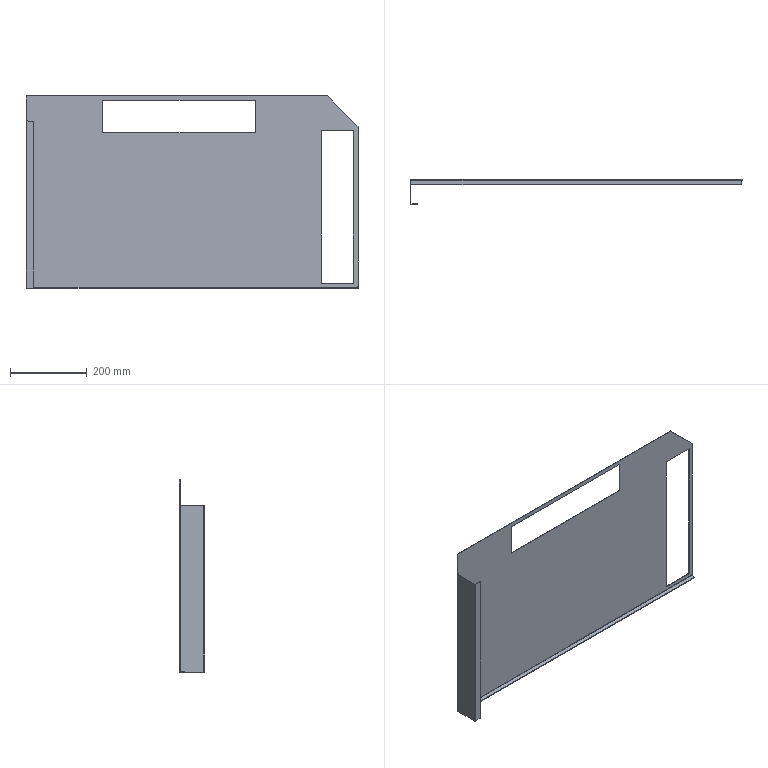Part | STEP file | Top Cover 2 | 1 solid | 39 faces | box 868 x 66 x 502.5 mm | volume 820735 mm3 | plane 30 | cylinder 9 | commonest cylinder face diameters 1 x6 5 x3
STEP:
#1=CARTESIAN_POINT('',(446.808,-2.,-297.25));
#2=VERTEX_POINT('',#1);
#3=CARTESIAN_POINT('',(447.308,-2.,-297.75));
#4=VERTEX_POINT('',#3);
#5=CARTESIAN_POINT('',(446.808,-2.,-297.75));
#6=DIRECTION('',(0.,1.,0.));
#7=DIRECTION('',(0.,0.,1.));
#8=AXIS2_PLACEMENT_3D('',#5,#6,#7);
#9=CIRCLE('',#8,0.5);
#10=EDGE_CURVE('',#2,#4,#9,.T.);
#11=ORIENTED_EDGE('',*,*,#10,.F.);
#12=CARTESIAN_POINT('',(446.808,0.,-297.25));
#13=VERTEX_POINT('',#12);
#14=CARTESIAN_POINT('',(446.808,-2.,-297.25));
#15=DIRECTION('',(0.,1.,0.));
#16=VECTOR('',#15,1000.);
#17=LINE('',#14,#16);
#18=EDGE_CURVE('',#2,#13,#17,.T.);
#19=ORIENTED_EDGE('',*,*,#18,.T.);
#20=CARTESIAN_POINT('',(447.308,0.,-297.75));
#21=VERTEX_POINT('',#20);
#22=CARTESIAN_POINT('',(446.808,0.,-297.75));
#23=DIRECTION('',(0.,-1.,0.));
#24=DIRECTION('',(0.,0.,1.));
#25=AXIS2_PLACEMENT_3D('',#22,#23,#24);
#26=CIRCLE('',#25,0.5);
#27=EDGE_CURVE('',#21,#13,#26,.T.);
#28=ORIENTED_EDGE('',*,*,#27,.F.);
#29=CARTESIAN_POINT('',(447.308,-2.,-297.75));
#30=DIRECTION('',(0.,1.,0.));
#31=VECTOR('',#30,1000.);
#32=LINE('',#29,#31);
#33=EDGE_CURVE('',#4,#21,#32,.T.);
#34=ORIENTED_EDGE('',*,*,#33,.F.);
#35=EDGE_LOOP('',(#11,#19,#28,#34));
#36=FACE_OUTER_BOUND('',#35,.T.);
#37=CARTESIAN_POINT('',(446.808,-2.,-297.75));
#38=DIRECTION('',(0.,1.,0.));
#39=DIRECTION('',(0.,0.,1.));
#40=AXIS2_PLACEMENT_3D('',#37,#38,#39);
#41=CYLINDRICAL_SURFACE('',#40,0.5);
#42=ADVANCED_FACE('',(#36),#41,.F.);
#43=ORIENTED_EDGE('',*,*,#27,.T.);
#44=CARTESIAN_POINT('',(446.308,0.,-297.75));
#45=VERTEX_POINT('',#44);
#46=CARTESIAN_POINT('',(446.808,0.,-297.75));
#47=DIRECTION('',(0.,-1.,0.));
#48=DIRECTION('',(0.,0.,1.));
#49=AXIS2_PLACEMENT_3D('',#46,#47,#48);
#50=CIRCLE('',#49,0.5);
#51=EDGE_CURVE('',#13,#45,#50,.T.);
#52=ORIENTED_EDGE('',*,*,#51,.T.);
#53=CARTESIAN_POINT('',(446.308,0.,-298.75));
#54=VERTEX_POINT('',#53);
#55=CARTESIAN_POINT('',(446.308,0.,-297.75));
#56=DIRECTION('',(0.,0.,1.));
#57=VECTOR('',#56,1000.);
#58=LINE('',#55,#57);
#59=EDGE_CURVE('',#54,#45,#58,.T.);
#60=ORIENTED_EDGE('',*,*,#59,.F.);
#61=CARTESIAN_POINT('',(-417.192,0.,-298.75));
#62=VERTEX_POINT('',#61);
#63=CARTESIAN_POINT('',(0.,0.,-298.75));
#64=DIRECTION('',(1.,0.,0.));
#65=VECTOR('',#64,1000.);
#66=LINE('',#63,#65);
#67=EDGE_CURVE('',#62,#54,#66,.T.);
#68=ORIENTED_EDGE('',*,*,#67,.F.);
#69=CARTESIAN_POINT('',(-417.192,0.,135.25));
#70=VERTEX_POINT('',#69);
#71=CARTESIAN_POINT('',(-417.192,0.,0.));
#72=DIRECTION('',(0.,0.,-1.));
#73=VECTOR('',#72,1000.);
#74=LINE('',#71,#73);
#75=EDGE_CURVE('',#70,#62,#74,.T.);
#76=ORIENTED_EDGE('',*,*,#75,.F.);
#77=CARTESIAN_POINT('',(-416.192,0.,135.25));
#78=VERTEX_POINT('',#77);
#79=CARTESIAN_POINT('',(-417.192,0.,135.25));
#80=DIRECTION('',(-1.,0.,0.));
#81=VECTOR('',#80,1000.);
#82=LINE('',#79,#81);
#83=EDGE_CURVE('',#78,#70,#82,.T.);
#84=ORIENTED_EDGE('',*,*,#83,.F.);
#85=CARTESIAN_POINT('',(-416.192,0.,136.25));
#86=VERTEX_POINT('',#85);
#87=CARTESIAN_POINT('',(-416.192,0.,135.75));
#88=DIRECTION('',(0.,-1.,0.));
#89=DIRECTION('',(0.,0.,1.));
#90=AXIS2_PLACEMENT_3D('',#87,#88,#89);
#91=CIRCLE('',#90,0.5);
#92=EDGE_CURVE('',#78,#86,#91,.T.);
#93=ORIENTED_EDGE('',*,*,#92,.T.);
#94=CARTESIAN_POINT('',(-419.692,0.,136.25));
#95=VERTEX_POINT('',#94);
#96=CARTESIAN_POINT('',(0.,0.,136.25));
#97=DIRECTION('',(1.,0.,0.));
#98=VECTOR('',#97,1000.);
#99=LINE('',#96,#98);
#100=EDGE_CURVE('',#95,#86,#99,.T.);
#101=ORIENTED_EDGE('',*,*,#100,.F.);
#102=CARTESIAN_POINT('',(-419.692,0.,201.25));
#103=VERTEX_POINT('',#102);
#104=CARTESIAN_POINT('',(-419.692,0.,0.));
#105=DIRECTION('',(0.,0.,-1.));
#106=VECTOR('',#105,1000.);
#107=LINE('',#104,#106);
#108=EDGE_CURVE('',#103,#95,#107,.T.);
#109=ORIENTED_EDGE('',*,*,#108,.F.);
#110=CARTESIAN_POINT('',(368.308,0.,201.25));
#111=VERTEX_POINT('',#110);
#112=CARTESIAN_POINT('',(0.,0.,201.25));
#113=DIRECTION('',(-1.,0.,0.));
#114=VECTOR('',#113,1000.);
#115=LINE('',#112,#114);
#116=EDGE_CURVE('',#111,#103,#115,.T.);
#117=ORIENTED_EDGE('',*,*,#116,.F.);
#118=CARTESIAN_POINT('',(448.308,0.,121.25));
#119=VERTEX_POINT('',#118);
#120=CARTESIAN_POINT('',(448.308,0.,121.25));
#121=DIRECTION('',(-0.7071,0.,0.7071));
#122=VECTOR('',#121,1000.);
#123=LINE('',#120,#122);
#124=EDGE_CURVE('',#119,#111,#123,.T.);
#125=ORIENTED_EDGE('',*,*,#124,.F.);
#126=CARTESIAN_POINT('',(448.308,0.,-301.25));
#127=VERTEX_POINT('',#126);
#128=CARTESIAN_POINT('',(448.308,0.,0.));
#129=DIRECTION('',(0.,0.,1.));
#130=VECTOR('',#129,1000.);
#131=LINE('',#128,#130);
#132=EDGE_CURVE('',#127,#119,#131,.T.);
#133=ORIENTED_EDGE('',*,*,#132,.F.);
#134=CARTESIAN_POINT('',(447.308,0.,-301.25));
#135=VERTEX_POINT('',#134);
#136=CARTESIAN_POINT('',(448.308,0.,-301.25));
#137=DIRECTION('',(1.,0.,0.));
#138=VECTOR('',#137,1000.);
#139=LINE('',#136,#138);
#140=EDGE_CURVE('',#135,#127,#139,.T.);
#141=ORIENTED_EDGE('',*,*,#140,.F.);
#142=CARTESIAN_POINT('',(447.308,0.,0.));
#143=DIRECTION('',(0.,0.,-1.));
#144=VECTOR('',#143,1000.);
#145=LINE('',#142,#144);
#146=EDGE_CURVE('',#21,#135,#145,.T.);
#147=ORIENTED_EDGE('',*,*,#146,.F.);
#148=EDGE_LOOP('',(#43,#52,#60,#68,#76,#84,#93,#101,#109,#117,#125,#133,#141,#147));
#149=FACE_OUTER_BOUND('',#148,.T.);
#150=CARTESIAN_POINT('',(-219.692,0.,105.25));
#151=VERTEX_POINT('',#150);
#152=CARTESIAN_POINT('',(-219.692,0.,189.25));
#153=VERTEX_POINT('',#152);
#154=CARTESIAN_POINT('',(-219.692,0.,0.));
#155=DIRECTION('',(0.,0.,1.));
#156=VECTOR('',#155,1000.);
#157=LINE('',#154,#156);
#158=EDGE_CURVE('',#151,#153,#157,.T.);
#159=ORIENTED_EDGE('',*,*,#158,.F.);
#160=CARTESIAN_POINT('',(180.308,0.,105.25));
#161=VERTEX_POINT('',#160);
#162=CARTESIAN_POINT('',(0.,0.,105.25));
#163=DIRECTION('',(-1.,0.,0.));
#164=VECTOR('',#163,1000.);
#165=LINE('',#162,#164);
#166=EDGE_CURVE('',#161,#151,#165,.T.);
#167=ORIENTED_EDGE('',*,*,#166,.F.);
#168=CARTESIAN_POINT('',(180.308,0.,189.25));
#169=VERTEX_POINT('',#168);
#170=CARTESIAN_POINT('',(180.308,0.,0.));
#171=DIRECTION('',(0.,0.,-1.));
#172=VECTOR('',#171,1000.);
#173=LINE('',#170,#172);
#174=EDGE_CURVE('',#169,#161,#173,.T.);
#175=ORIENTED_EDGE('',*,*,#174,.F.);
#176=CARTESIAN_POINT('',(0.,0.,189.25));
#177=DIRECTION('',(1.,0.,0.));
#178=VECTOR('',#177,1000.);
#179=LINE('',#176,#178);
#180=EDGE_CURVE('',#153,#169,#179,.T.);
#181=ORIENTED_EDGE('',*,*,#180,.F.);
#182=EDGE_LOOP('',(#159,#167,#175,#181));
#183=FACE_BOUND('',#182,.T.);
#184=CARTESIAN_POINT('',(352.308,0.,-288.75));
#185=VERTEX_POINT('',#184);
#186=CARTESIAN_POINT('',(352.308,0.,111.25));
#187=VERTEX_POINT('',#186);
#188=CARTESIAN_POINT('',(352.308,0.,0.));
#189=DIRECTION('',(0.,0.,1.));
#190=VECTOR('',#189,1000.);
#191=LINE('',#188,#190);
#192=EDGE_CURVE('',#185,#187,#191,.T.);
#193=ORIENTED_EDGE('',*,*,#192,.F.);
#194=CARTESIAN_POINT('',(436.308,0.,-288.75));
#195=VERTEX_POINT('',#194);
#196=CARTESIAN_POINT('',(0.,0.,-288.75));
#197=DIRECTION('',(-1.,0.,0.));
#198=VECTOR('',#197,1000.);
#199=LINE('',#196,#198);
#200=EDGE_CURVE('',#195,#185,#199,.T.);
#201=ORIENTED_EDGE('',*,*,#200,.F.);
#202=CARTESIAN_POINT('',(436.308,0.,111.25));
#203=VERTEX_POINT('',#202);
#204=CARTESIAN_POINT('',(436.308,0.,0.));
#205=DIRECTION('',(0.,0.,-1.));
#206=VECTOR('',#205,1000.);
#207=LINE('',#204,#206);
#208=EDGE_CURVE('',#203,#195,#207,.T.);
#209=ORIENTED_EDGE('',*,*,#208,.F.);
#210=CARTESIAN_POINT('',(0.,0.,111.25));
#211=DIRECTION('',(1.,0.,0.));
#212=VECTOR('',#211,1000.);
#213=LINE('',#210,#212);
#214=EDGE_CURVE('',#187,#203,#213,.T.);
#215=ORIENTED_EDGE('',*,*,#214,.F.);
#216=EDGE_LOOP('',(#193,#201,#209,#215));
#217=FACE_BOUND('',#216,.T.);
#218=CARTESIAN_POINT('',(0.,0.,0.));
#219=DIRECTION('',(0.,-1.,0.));
#220=DIRECTION('',(0.,0.,-1.));
#221=AXIS2_PLACEMENT_3D('',#218,#219,#220);
#222=PLANE('',#221);
#223=ADVANCED_FACE('',(#149,#183,#217),#222,.F.);
#224=CARTESIAN_POINT('',(447.308,-2.,-301.25));
#225=VERTEX_POINT('',#224);
#226=CARTESIAN_POINT('',(447.308,-2.,-301.25));
#227=DIRECTION('',(0.,-1.,0.));
#228=VECTOR('',#227,1000.);
#229=LINE('',#226,#228);
#230=EDGE_CURVE('',#135,#225,#229,.T.);
#231=ORIENTED_EDGE('',*,*,#230,.T.);
#232=CARTESIAN_POINT('',(447.308,-2.,-301.25));
#233=DIRECTION('',(0.,0.,1.));
#234=VECTOR('',#233,1000.);
#235=LINE('',#232,#234);
#236=EDGE_CURVE('',#225,#4,#235,.T.);
#237=ORIENTED_EDGE('',*,*,#236,.T.);
#238=ORIENTED_EDGE('',*,*,#33,.T.);
#239=ORIENTED_EDGE('',*,*,#146,.T.);
#240=EDGE_LOOP('',(#231,#237,#238,#239));
#241=FACE_OUTER_BOUND('',#240,.T.);
#242=CARTESIAN_POINT('',(447.308,-2.,-301.25));
#243=DIRECTION('',(-1.,0.,0.));
#244=DIRECTION('',(0.,0.,1.));
#245=AXIS2_PLACEMENT_3D('',#242,#243,#244);
#246=PLANE('',#245);
#247=ADVANCED_FACE('',(#241),#246,.T.);
#248=CARTESIAN_POINT('',(-417.192,-2.,-301.199));
#249=VERTEX_POINT('',#248);
#250=CARTESIAN_POINT('',(-417.192,-2.5,-301.25));
#251=VERTEX_POINT('',#250);
#252=CARTESIAN_POINT('',(-417.192,-2.5,-298.75));
#253=DIRECTION('',(-1.,0.,0.));
#254=DIRECTION('',(0.,0.,-1.));
#255=AXIS2_PLACEMENT_3D('',#252,#253,#254);
#256=CIRCLE('',#255,2.5);
#257=EDGE_CURVE('',#249,#251,#256,.T.);
#258=ORIENTED_EDGE('',*,*,#257,.F.);
#259=CARTESIAN_POINT('',(-417.192,-2.5,-298.75));
#260=DIRECTION('',(1.,0.,0.));
#261=DIRECTION('',(0.,0.,-1.));
#262=AXIS2_PLACEMENT_3D('',#259,#260,#261);
#263=CIRCLE('',#262,2.5);
#264=EDGE_CURVE('',#249,#62,#263,.T.);
#265=ORIENTED_EDGE('',*,*,#264,.T.);
#266=ORIENTED_EDGE('',*,*,#67,.T.);
#267=CARTESIAN_POINT('',(446.308,-2.5,-301.25));
#268=VERTEX_POINT('',#267);
#269=CARTESIAN_POINT('',(446.308,-2.5,-298.75));
#270=DIRECTION('',(-1.,0.,0.));
#271=DIRECTION('',(0.,0.,-1.));
#272=AXIS2_PLACEMENT_3D('',#269,#270,#271);
#273=CIRCLE('',#272,2.5);
#274=EDGE_CURVE('',#54,#268,#273,.T.);
#275=ORIENTED_EDGE('',*,*,#274,.T.);
#276=CARTESIAN_POINT('',(446.308,-2.5,-301.25));
#277=DIRECTION('',(-1.,0.,0.));
#278=VECTOR('',#277,1000.);
#279=LINE('',#276,#278);
#280=EDGE_CURVE('',#268,#251,#279,.T.);
#281=ORIENTED_EDGE('',*,*,#280,.T.);
#282=EDGE_LOOP('',(#258,#265,#266,#275,#281));
#283=FACE_OUTER_BOUND('',#282,.T.);
#284=CARTESIAN_POINT('',(446.308,-2.5,-298.75));
#285=DIRECTION('',(1.,0.,0.));
#286=DIRECTION('',(0.,0.,-1.));
#287=AXIS2_PLACEMENT_3D('',#284,#285,#286);
#288=CYLINDRICAL_SURFACE('',#287,2.5);
#289=ADVANCED_FACE('',(#283),#288,.T.);
#290=CARTESIAN_POINT('',(-419.692,-2.5,135.25));
#291=VERTEX_POINT('',#290);
#292=CARTESIAN_POINT('',(-417.192,-2.5,135.25));
#293=DIRECTION('',(0.,0.,-1.));
#294=DIRECTION('',(-1.,0.,0.));
#295=AXIS2_PLACEMENT_3D('',#292,#293,#294);
#296=CIRCLE('',#295,2.5);
#297=EDGE_CURVE('',#291,#70,#296,.T.);
#298=ORIENTED_EDGE('',*,*,#297,.T.);
#299=ORIENTED_EDGE('',*,*,#75,.T.);
#300=CARTESIAN_POINT('',(-417.192,0.,-301.25));
#301=VERTEX_POINT('',#300);
#302=CARTESIAN_POINT('',(-417.192,0.,-301.25));
#303=DIRECTION('',(0.,0.,-1.));
#304=VECTOR('',#303,1000.);
#305=LINE('',#302,#304);
#306=EDGE_CURVE('',#62,#301,#305,.T.);
#307=ORIENTED_EDGE('',*,*,#306,.T.);
#308=CARTESIAN_POINT('',(-419.692,-2.5,-301.25));
#309=VERTEX_POINT('',#308);
#310=CARTESIAN_POINT('',(-417.192,-2.5,-301.25));
#311=DIRECTION('',(0.,0.,1.));
#312=DIRECTION('',(-1.,0.,0.));
#313=AXIS2_PLACEMENT_3D('',#310,#311,#312);
#314=CIRCLE('',#313,2.5);
#315=EDGE_CURVE('',#301,#309,#314,.T.);
#316=ORIENTED_EDGE('',*,*,#315,.T.);
#317=CARTESIAN_POINT('',(-419.692,-2.5,-301.25));
#318=DIRECTION('',(0.,0.,1.));
#319=VECTOR('',#318,1000.);
#320=LINE('',#317,#319);
#321=EDGE_CURVE('',#309,#291,#320,.T.);
#322=ORIENTED_EDGE('',*,*,#321,.T.);
#323=EDGE_LOOP('',(#298,#299,#307,#316,#322));
#324=FACE_OUTER_BOUND('',#323,.T.);
#325=CARTESIAN_POINT('',(-417.192,-2.5,-301.25));
#326=DIRECTION('',(0.,0.,-1.));
#327=DIRECTION('',(-1.,0.,0.));
#328=AXIS2_PLACEMENT_3D('',#325,#326,#327);
#329=CYLINDRICAL_SURFACE('',#328,2.5);
#330=ADVANCED_FACE('',(#324),#329,.T.);
#331=CARTESIAN_POINT('',(-416.192,-2.,136.25));
#332=VERTEX_POINT('',#331);
#333=CARTESIAN_POINT('',(-416.192,-2.,136.25));
#334=DIRECTION('',(0.,-1.,0.));
#335=VECTOR('',#334,1000.);
#336=LINE('',#333,#335);
#337=EDGE_CURVE('',#86,#332,#336,.T.);
#338=ORIENTED_EDGE('',*,*,#337,.T.);
#339=CARTESIAN_POINT('',(-419.692,-2.,136.25));
#340=VERTEX_POINT('',#339);
#341=CARTESIAN_POINT('',(-416.192,-2.,136.25));
#342=DIRECTION('',(-1.,0.,0.));
#343=VECTOR('',#342,1000.);
#344=LINE('',#341,#343);
#345=EDGE_CURVE('',#332,#340,#344,.T.);
#346=ORIENTED_EDGE('',*,*,#345,.T.);
#347=CARTESIAN_POINT('',(-419.692,-2.,136.25));
#348=DIRECTION('',(0.,1.,0.));
#349=VECTOR('',#348,1000.);
#350=LINE('',#347,#349);
#351=EDGE_CURVE('',#340,#95,#350,.T.);
#352=ORIENTED_EDGE('',*,*,#351,.T.);
#353=ORIENTED_EDGE('',*,*,#100,.T.);
#354=EDGE_LOOP('',(#338,#346,#352,#353));
#355=FACE_OUTER_BOUND('',#354,.T.);
#356=CARTESIAN_POINT('',(-416.192,-2.,136.25));
#357=DIRECTION('',(0.,0.,-1.));
#358=DIRECTION('',(0.,1.,0.));
#359=AXIS2_PLACEMENT_3D('',#356,#357,#358);
#360=PLANE('',#359);
#361=ADVANCED_FACE('',(#355),#360,.T.);
#362=CARTESIAN_POINT('',(-419.692,-2.,201.25));
#363=VERTEX_POINT('',#362);
#364=CARTESIAN_POINT('',(-419.692,-2.,-301.25));
#365=DIRECTION('',(0.,0.,1.));
#366=VECTOR('',#365,1000.);
#367=LINE('',#364,#366);
#368=EDGE_CURVE('',#340,#363,#367,.T.);
#369=ORIENTED_EDGE('',*,*,#368,.T.);
#370=CARTESIAN_POINT('',(-419.692,-2.,201.25));
#371=DIRECTION('',(0.,1.,0.));
#372=VECTOR('',#371,1000.);
#373=LINE('',#370,#372);
#374=EDGE_CURVE('',#363,#103,#373,.T.);
#375=ORIENTED_EDGE('',*,*,#374,.T.);
#376=ORIENTED_EDGE('',*,*,#108,.T.);
#377=ORIENTED_EDGE('',*,*,#351,.F.);
#378=EDGE_LOOP('',(#369,#375,#376,#377));
#379=FACE_OUTER_BOUND('',#378,.T.);
#380=CARTESIAN_POINT('',(-419.692,-2.,-301.25));
#381=DIRECTION('',(-1.,0.,0.));
#382=DIRECTION('',(0.,0.,1.));
#383=AXIS2_PLACEMENT_3D('',#380,#381,#382);
#384=PLANE('',#383);
#385=ADVANCED_FACE('',(#379),#384,.T.);
#386=CARTESIAN_POINT('',(368.308,-2.,201.25));
#387=VERTEX_POINT('',#386);
#388=CARTESIAN_POINT('',(368.308,-2.,201.25));
#389=DIRECTION('',(1.,0.,0.));
#390=VECTOR('',#389,1000.);
#391=LINE('',#388,#390);
#392=EDGE_CURVE('',#363,#387,#391,.T.);
#393=ORIENTED_EDGE('',*,*,#392,.T.);
#394=CARTESIAN_POINT('',(368.308,-2.,201.25));
#395=DIRECTION('',(0.,1.,0.));
#396=VECTOR('',#395,1000.);
#397=LINE('',#394,#396);
#398=EDGE_CURVE('',#387,#111,#397,.T.);
#399=ORIENTED_EDGE('',*,*,#398,.T.);
#400=ORIENTED_EDGE('',*,*,#116,.T.);
#401=ORIENTED_EDGE('',*,*,#374,.F.);
#402=EDGE_LOOP('',(#393,#399,#400,#401));
#403=FACE_OUTER_BOUND('',#402,.T.);
#404=CARTESIAN_POINT('',(368.308,-2.,201.25));
#405=DIRECTION('',(0.,0.,1.));
#406=DIRECTION('',(1.,0.,0.));
#407=AXIS2_PLACEMENT_3D('',#404,#405,#406);
#408=PLANE('',#407);
#409=ADVANCED_FACE('',(#403),#408,.T.);
#410=CARTESIAN_POINT('',(448.308,-2.,121.25));
#411=VERTEX_POINT('',#410);
#412=CARTESIAN_POINT('',(448.308,-2.,121.25));
#413=DIRECTION('',(0.7071,0.,-0.7071));
#414=VECTOR('',#413,1000.);
#415=LINE('',#412,#414);
#416=EDGE_CURVE('',#387,#411,#415,.T.);
#417=ORIENTED_EDGE('',*,*,#416,.T.);
#418=CARTESIAN_POINT('',(448.308,-2.,121.25));
#419=DIRECTION('',(0.,1.,0.));
#420=VECTOR('',#419,1000.);
#421=LINE('',#418,#420);
#422=EDGE_CURVE('',#411,#119,#421,.T.);
#423=ORIENTED_EDGE('',*,*,#422,.T.);
#424=ORIENTED_EDGE('',*,*,#124,.T.);
#425=ORIENTED_EDGE('',*,*,#398,.F.);
#426=EDGE_LOOP('',(#417,#423,#424,#425));
#427=FACE_OUTER_BOUND('',#426,.T.);
#428=CARTESIAN_POINT('',(448.308,-2.,121.25));
#429=DIRECTION('',(0.7071,0.,0.7071));
#430=DIRECTION('',(0.7071,0.,-0.7071));
#431=AXIS2_PLACEMENT_3D('',#428,#429,#430);
#432=PLANE('',#431);
#433=ADVANCED_FACE('',(#427),#432,.T.);
#434=CARTESIAN_POINT('',(448.308,-2.,-301.25));
#435=VERTEX_POINT('',#434);
#436=CARTESIAN_POINT('',(448.308,-2.,-301.25));
#437=DIRECTION('',(0.,0.,-1.));
#438=VECTOR('',#437,1000.);
#439=LINE('',#436,#438);
#440=EDGE_CURVE('',#411,#435,#439,.T.);
#441=ORIENTED_EDGE('',*,*,#440,.T.);
#442=CARTESIAN_POINT('',(448.308,-2.,-301.25));
#443=DIRECTION('',(0.,1.,0.));
#444=VECTOR('',#443,1000.);
#445=LINE('',#442,#444);
#446=EDGE_CURVE('',#435,#127,#445,.T.);
#447=ORIENTED_EDGE('',*,*,#446,.T.);
#448=ORIENTED_EDGE('',*,*,#132,.T.);
#449=ORIENTED_EDGE('',*,*,#422,.F.);
#450=EDGE_LOOP('',(#441,#447,#448,#449));
#451=FACE_OUTER_BOUND('',#450,.T.);
#452=CARTESIAN_POINT('',(448.308,-2.,-301.25));
#453=DIRECTION('',(1.,0.,0.));
#454=DIRECTION('',(0.,0.,-1.));
#455=AXIS2_PLACEMENT_3D('',#452,#453,#454);
#456=PLANE('',#455);
#457=ADVANCED_FACE('',(#451),#456,.T.);
#458=CARTESIAN_POINT('',(-219.692,-2.,189.25));
#459=VERTEX_POINT('',#458);
#460=CARTESIAN_POINT('',(-219.692,-10.,189.25));
#461=DIRECTION('',(0.,-1.,0.));
#462=VECTOR('',#461,1000.);
#463=LINE('',#460,#462);
#464=EDGE_CURVE('',#153,#459,#463,.T.);
#465=ORIENTED_EDGE('',*,*,#464,.F.);
#466=ORIENTED_EDGE('',*,*,#180,.T.);
#467=CARTESIAN_POINT('',(180.308,-2.,189.25));
#468=VERTEX_POINT('',#467);
#469=CARTESIAN_POINT('',(180.308,-10.,189.25));
#470=DIRECTION('',(0.,1.,0.));
#471=VECTOR('',#470,1000.);
#472=LINE('',#469,#471);
#473=EDGE_CURVE('',#468,#169,#472,.T.);
#474=ORIENTED_EDGE('',*,*,#473,.F.);
#475=CARTESIAN_POINT('',(-219.692,-2.,189.25));
#476=DIRECTION('',(1.,0.,0.));
#477=VECTOR('',#476,1000.);
#478=LINE('',#475,#477);
#479=EDGE_CURVE('',#459,#468,#478,.T.);
#480=ORIENTED_EDGE('',*,*,#479,.F.);
#481=EDGE_LOOP('',(#465,#466,#474,#480));
#482=FACE_OUTER_BOUND('',#481,.T.);
#483=CARTESIAN_POINT('',(-219.692,-10.,189.25));
#484=DIRECTION('',(0.,0.,1.));
#485=DIRECTION('',(1.,0.,0.));
#486=AXIS2_PLACEMENT_3D('',#483,#484,#485);
#487=PLANE('',#486);
#488=ADVANCED_FACE('',(#482),#487,.F.);
#489=CARTESIAN_POINT('',(-219.692,-2.,105.25));
#490=VERTEX_POINT('',#489);
#491=CARTESIAN_POINT('',(-219.692,-10.,105.25));
#492=DIRECTION('',(0.,-1.,0.));
#493=VECTOR('',#492,1000.);
#494=LINE('',#491,#493);
#495=EDGE_CURVE('',#151,#490,#494,.T.);
#496=ORIENTED_EDGE('',*,*,#495,.F.);
#497=ORIENTED_EDGE('',*,*,#158,.T.);
#498=ORIENTED_EDGE('',*,*,#464,.T.);
#499=CARTESIAN_POINT('',(-219.692,-2.,105.25));
#500=DIRECTION('',(0.,0.,1.));
#501=VECTOR('',#500,1000.);
#502=LINE('',#499,#501);
#503=EDGE_CURVE('',#490,#459,#502,.T.);
#504=ORIENTED_EDGE('',*,*,#503,.F.);
#505=EDGE_LOOP('',(#496,#497,#498,#504));
#506=FACE_OUTER_BOUND('',#505,.T.);
#507=CARTESIAN_POINT('',(-219.692,-10.,105.25));
#508=DIRECTION('',(-1.,0.,0.));
#509=DIRECTION('',(0.,0.,1.));
#510=AXIS2_PLACEMENT_3D('',#507,#508,#509);
#511=PLANE('',#510);
#512=ADVANCED_FACE('',(#506),#511,.F.);
#513=CARTESIAN_POINT('',(180.308,-2.,105.25));
#514=VERTEX_POINT('',#513);
#515=CARTESIAN_POINT('',(180.308,-10.,105.25));
#516=DIRECTION('',(0.,-1.,0.));
#517=VECTOR('',#516,1000.);
#518=LINE('',#515,#517);
#519=EDGE_CURVE('',#161,#514,#518,.T.);
#520=ORIENTED_EDGE('',*,*,#519,.F.);
#521=ORIENTED_EDGE('',*,*,#166,.T.);
#522=ORIENTED_EDGE('',*,*,#495,.T.);
#523=CARTESIAN_POINT('',(-219.692,-2.,105.25));
#524=DIRECTION('',(-1.,0.,0.));
#525=VECTOR('',#524,1000.);
#526=LINE('',#523,#525);
#527=EDGE_CURVE('',#514,#490,#526,.T.);
#528=ORIENTED_EDGE('',*,*,#527,.F.);
#529=EDGE_LOOP('',(#520,#521,#522,#528));
#530=FACE_OUTER_BOUND('',#529,.T.);
#531=CARTESIAN_POINT('',(-219.692,-10.,105.25));
#532=DIRECTION('',(0.,0.,-1.));
#533=DIRECTION('',(-1.,0.,0.));
#534=AXIS2_PLACEMENT_3D('',#531,#532,#533);
#535=PLANE('',#534);
#536=ADVANCED_FACE('',(#530),#535,.F.);
#537=ORIENTED_EDGE('',*,*,#473,.T.);
#538=ORIENTED_EDGE('',*,*,#174,.T.);
#539=ORIENTED_EDGE('',*,*,#519,.T.);
#540=CARTESIAN_POINT('',(180.308,-2.,105.25));
#541=DIRECTION('',(0.,0.,-1.));
#542=VECTOR('',#541,1000.);
#543=LINE('',#540,#542);
#544=EDGE_CURVE('',#468,#514,#543,.T.);
#545=ORIENTED_EDGE('',*,*,#544,.F.);
#546=EDGE_LOOP('',(#537,#538,#539,#545));
#547=FACE_OUTER_BOUND('',#546,.T.);
#548=CARTESIAN_POINT('',(180.308,-10.,105.25));
#549=DIRECTION('',(1.,0.,0.));
#550=DIRECTION('',(0.,0.,-1.));
#551=AXIS2_PLACEMENT_3D('',#548,#549,#550);
#552=PLANE('',#551);
#553=ADVANCED_FACE('',(#547),#552,.F.);
#554=CARTESIAN_POINT('',(352.308,-2.,111.25));
#555=VERTEX_POINT('',#554);
#556=CARTESIAN_POINT('',(352.308,-10.,111.25));
#557=DIRECTION('',(0.,-1.,0.));
#558=VECTOR('',#557,1000.);
#559=LINE('',#556,#558);
#560=EDGE_CURVE('',#187,#555,#559,.T.);
#561=ORIENTED_EDGE('',*,*,#560,.F.);
#562=ORIENTED_EDGE('',*,*,#214,.T.);
#563=CARTESIAN_POINT('',(436.308,-2.,111.25));
#564=VERTEX_POINT('',#563);
#565=CARTESIAN_POINT('',(436.308,-10.,111.25));
#566=DIRECTION('',(0.,1.,0.));
#567=VECTOR('',#566,1000.);
#568=LINE('',#565,#567);
#569=EDGE_CURVE('',#564,#203,#568,.T.);
#570=ORIENTED_EDGE('',*,*,#569,.F.);
#571=CARTESIAN_POINT('',(352.308,-2.,111.25));
#572=DIRECTION('',(1.,0.,0.));
#573=VECTOR('',#572,1000.);
#574=LINE('',#571,#573);
#575=EDGE_CURVE('',#555,#564,#574,.T.);
#576=ORIENTED_EDGE('',*,*,#575,.F.);
#577=EDGE_LOOP('',(#561,#562,#570,#576));
#578=FACE_OUTER_BOUND('',#577,.T.);
#579=CARTESIAN_POINT('',(352.308,-10.,111.25));
#580=DIRECTION('',(0.,0.,1.));
#581=DIRECTION('',(1.,0.,0.));
#582=AXIS2_PLACEMENT_3D('',#579,#580,#581);
#583=PLANE('',#582);
#584=ADVANCED_FACE('',(#578),#583,.F.);
#585=CARTESIAN_POINT('',(352.308,-2.,-288.75));
#586=VERTEX_POINT('',#585);
#587=CARTESIAN_POINT('',(352.308,-10.,-288.75));
#588=DIRECTION('',(0.,-1.,0.));
#589=VECTOR('',#588,1000.);
#590=LINE('',#587,#589);
#591=EDGE_CURVE('',#185,#586,#590,.T.);
#592=ORIENTED_EDGE('',*,*,#591,.F.);
#593=ORIENTED_EDGE('',*,*,#192,.T.);
#594=ORIENTED_EDGE('',*,*,#560,.T.);
#595=CARTESIAN_POINT('',(352.308,-2.,-288.75));
#596=DIRECTION('',(0.,0.,1.));
#597=VECTOR('',#596,1000.);
#598=LINE('',#595,#597);
#599=EDGE_CURVE('',#586,#555,#598,.T.);
#600=ORIENTED_EDGE('',*,*,#599,.F.);
#601=EDGE_LOOP('',(#592,#593,#594,#600));
#602=FACE_OUTER_BOUND('',#601,.T.);
#603=CARTESIAN_POINT('',(352.308,-10.,-288.75));
#604=DIRECTION('',(-1.,0.,0.));
#605=DIRECTION('',(0.,0.,1.));
#606=AXIS2_PLACEMENT_3D('',#603,#604,#605);
#607=PLANE('',#606);
#608=ADVANCED_FACE('',(#602),#607,.F.);
#609=CARTESIAN_POINT('',(436.308,-2.,-288.75));
#610=VERTEX_POINT('',#609);
#611=CARTESIAN_POINT('',(436.308,-10.,-288.75));
#612=DIRECTION('',(0.,-1.,0.));
#613=VECTOR('',#612,1000.);
#614=LINE('',#611,#613);
#615=EDGE_CURVE('',#195,#610,#614,.T.);
#616=ORIENTED_EDGE('',*,*,#615,.F.);
#617=ORIENTED_EDGE('',*,*,#200,.T.);
#618=ORIENTED_EDGE('',*,*,#591,.T.);
#619=CARTESIAN_POINT('',(352.308,-2.,-288.75));
#620=DIRECTION('',(-1.,0.,0.));
#621=VECTOR('',#620,1000.);
#622=LINE('',#619,#621);
#623=EDGE_CURVE('',#610,#586,#622,.T.);
#624=ORIENTED_EDGE('',*,*,#623,.F.);
#625=EDGE_LOOP('',(#616,#617,#618,#624));
#626=FACE_OUTER_BOUND('',#625,.T.);
#627=CARTESIAN_POINT('',(352.308,-10.,-288.75));
#628=DIRECTION('',(0.,0.,-1.));
#629=DIRECTION('',(-1.,0.,0.));
#630=AXIS2_PLACEMENT_3D('',#627,#628,#629);
#631=PLANE('',#630);
#632=ADVANCED_FACE('',(#626),#631,.F.);
#633=ORIENTED_EDGE('',*,*,#569,.T.);
#634=ORIENTED_EDGE('',*,*,#208,.T.);
#635=ORIENTED_EDGE('',*,*,#615,.T.);
#636=CARTESIAN_POINT('',(436.308,-2.,-288.75));
#637=DIRECTION('',(0.,0.,-1.));
#638=VECTOR('',#637,1000.);
#639=LINE('',#636,#638);
#640=EDGE_CURVE('',#564,#610,#639,.T.);
#641=ORIENTED_EDGE('',*,*,#640,.F.);
#642=EDGE_LOOP('',(#633,#634,#635,#641));
#643=FACE_OUTER_BOUND('',#642,.T.);
#644=CARTESIAN_POINT('',(436.308,-10.,-288.75));
#645=DIRECTION('',(1.,0.,0.));
#646=DIRECTION('',(0.,0.,-1.));
#647=AXIS2_PLACEMENT_3D('',#644,#645,#646);
#648=PLANE('',#647);
#649=ADVANCED_FACE('',(#643),#648,.F.);
#650=CARTESIAN_POINT('',(446.308,-2.,-297.75));
#651=VERTEX_POINT('',#650);
#652=CARTESIAN_POINT('',(446.308,-2.,-298.75));
#653=VERTEX_POINT('',#652);
#654=CARTESIAN_POINT('',(446.308,-2.,-297.75));
#655=DIRECTION('',(0.,0.,-1.));
#656=VECTOR('',#655,1000.);
#657=LINE('',#654,#656);
#658=EDGE_CURVE('',#651,#653,#657,.T.);
#659=ORIENTED_EDGE('',*,*,#658,.F.);
#660=CARTESIAN_POINT('',(446.808,-2.,-297.75));
#661=DIRECTION('',(0.,1.,0.));
#662=DIRECTION('',(0.,0.,1.));
#663=AXIS2_PLACEMENT_3D('',#660,#661,#662);
#664=CIRCLE('',#663,0.5);
#665=EDGE_CURVE('',#651,#2,#664,.T.);
#666=ORIENTED_EDGE('',*,*,#665,.T.);
#667=ORIENTED_EDGE('',*,*,#10,.T.);
#668=ORIENTED_EDGE('',*,*,#236,.F.);
#669=CARTESIAN_POINT('',(0.,-2.,-301.25));
#670=DIRECTION('',(1.,0.,0.));
#671=VECTOR('',#670,1000.);
#672=LINE('',#669,#671);
#673=EDGE_CURVE('',#225,#435,#672,.T.);
#674=ORIENTED_EDGE('',*,*,#673,.T.);
#675=ORIENTED_EDGE('',*,*,#440,.F.);
#676=ORIENTED_EDGE('',*,*,#416,.F.);
#677=ORIENTED_EDGE('',*,*,#392,.F.);
#678=ORIENTED_EDGE('',*,*,#368,.F.);
#679=ORIENTED_EDGE('',*,*,#345,.F.);
#680=CARTESIAN_POINT('',(-416.192,-2.,135.25));
#681=VERTEX_POINT('',#680);
#682=CARTESIAN_POINT('',(-416.192,-2.,135.75));
#683=DIRECTION('',(0.,1.,0.));
#684=DIRECTION('',(0.,0.,1.));
#685=AXIS2_PLACEMENT_3D('',#682,#683,#684);
#686=CIRCLE('',#685,0.5);
#687=EDGE_CURVE('',#332,#681,#686,.T.);
#688=ORIENTED_EDGE('',*,*,#687,.T.);
#689=CARTESIAN_POINT('',(-417.192,-2.,135.25));
#690=VERTEX_POINT('',#689);
#691=CARTESIAN_POINT('',(-417.192,-2.,135.25));
#692=DIRECTION('',(1.,0.,0.));
#693=VECTOR('',#692,1000.);
#694=LINE('',#691,#693);
#695=EDGE_CURVE('',#690,#681,#694,.T.);
#696=ORIENTED_EDGE('',*,*,#695,.F.);
#697=CARTESIAN_POINT('',(-417.192,-2.,-298.75));
#698=VERTEX_POINT('',#697);
#699=CARTESIAN_POINT('',(-417.192,-2.,0.));
#700=DIRECTION('',(0.,0.,-1.));
#701=VECTOR('',#700,1000.);
#702=LINE('',#699,#701);
#703=EDGE_CURVE('',#690,#698,#702,.T.);
#704=ORIENTED_EDGE('',*,*,#703,.T.);
#705=CARTESIAN_POINT('',(0.,-2.,-298.75));
#706=DIRECTION('',(1.,0.,0.));
#707=VECTOR('',#706,1000.);
#708=LINE('',#705,#707);
#709=EDGE_CURVE('',#698,#653,#708,.T.);
#710=ORIENTED_EDGE('',*,*,#709,.T.);
#711=EDGE_LOOP('',(#659,#666,#667,#668,#674,#675,#676,#677,#678,#679,#688,#696,#704,#710));
#712=FACE_OUTER_BOUND('',#711,.T.);
#713=ORIENTED_EDGE('',*,*,#544,.T.);
#714=ORIENTED_EDGE('',*,*,#527,.T.);
#715=ORIENTED_EDGE('',*,*,#503,.T.);
#716=ORIENTED_EDGE('',*,*,#479,.T.);
#717=EDGE_LOOP('',(#713,#714,#715,#716));
#718=FACE_BOUND('',#717,.T.);
#719=ORIENTED_EDGE('',*,*,#640,.T.);
#720=ORIENTED_EDGE('',*,*,#623,.T.);
#721=ORIENTED_EDGE('',*,*,#599,.T.);
#722=ORIENTED_EDGE('',*,*,#575,.T.);
#723=EDGE_LOOP('',(#719,#720,#721,#722));
#724=FACE_BOUND('',#723,.T.);
#725=CARTESIAN_POINT('',(0.,-2.,0.));
#726=DIRECTION('',(0.,-1.,0.));
#727=DIRECTION('',(0.,0.,-1.));
#728=AXIS2_PLACEMENT_3D('',#725,#726,#727);
#729=PLANE('',#728);
#730=ADVANCED_FACE('',(#712,#718,#724),#729,.T.);
#731=ORIENTED_EDGE('',*,*,#140,.T.);
#732=ORIENTED_EDGE('',*,*,#446,.F.);
#733=ORIENTED_EDGE('',*,*,#673,.F.);
#734=ORIENTED_EDGE('',*,*,#230,.F.);
#735=EDGE_LOOP('',(#731,#732,#733,#734));
#736=FACE_OUTER_BOUND('',#735,.T.);
#737=CARTESIAN_POINT('',(448.308,-2.,-301.25));
#738=DIRECTION('',(0.,0.,-1.));
#739=DIRECTION('',(-1.,0.,0.));
#740=AXIS2_PLACEMENT_3D('',#737,#738,#739);
#741=PLANE('',#740);
#742=ADVANCED_FACE('',(#736),#741,.T.);
#743=ORIENTED_EDGE('',*,*,#18,.F.);
#744=ORIENTED_EDGE('',*,*,#665,.F.);
#745=CARTESIAN_POINT('',(446.308,-2.,-297.75));
#746=DIRECTION('',(0.,-1.,0.));
#747=VECTOR('',#746,1000.);
#748=LINE('',#745,#747);
#749=EDGE_CURVE('',#45,#651,#748,.T.);
#750=ORIENTED_EDGE('',*,*,#749,.F.);
#751=ORIENTED_EDGE('',*,*,#51,.F.);
#752=EDGE_LOOP('',(#743,#744,#750,#751));
#753=FACE_OUTER_BOUND('',#752,.T.);
#754=CARTESIAN_POINT('',(446.808,-2.,-297.75));
#755=DIRECTION('',(0.,1.,0.));
#756=DIRECTION('',(0.,0.,1.));
#757=AXIS2_PLACEMENT_3D('',#754,#755,#756);
#758=CYLINDRICAL_SURFACE('',#757,0.5);
#759=ADVANCED_FACE('',(#753),#758,.F.);
#760=CARTESIAN_POINT('',(-417.192,-2.,-301.25));
#761=VERTEX_POINT('',#760);
#762=CARTESIAN_POINT('',(-417.192,-2.,-298.75));
#763=DIRECTION('',(0.,0.,-1.));
#764=VECTOR('',#763,1000.);
#765=LINE('',#762,#764);
#766=EDGE_CURVE('',#249,#761,#765,.T.);
#767=ORIENTED_EDGE('',*,*,#766,.T.);
#768=CARTESIAN_POINT('',(-417.192,-2.,-301.25));
#769=DIRECTION('',(0.,1.,0.));
#770=VECTOR('',#769,1000.);
#771=LINE('',#768,#770);
#772=EDGE_CURVE('',#761,#301,#771,.T.);
#773=ORIENTED_EDGE('',*,*,#772,.T.);
#774=ORIENTED_EDGE('',*,*,#306,.F.);
#775=ORIENTED_EDGE('',*,*,#264,.F.);
#776=EDGE_LOOP('',(#767,#773,#774,#775));
#777=FACE_OUTER_BOUND('',#776,.T.);
#778=CARTESIAN_POINT('',(-417.192,-2.,-298.75));
#779=DIRECTION('',(1.,0.,0.));
#780=DIRECTION('',(0.,0.,-1.));
#781=AXIS2_PLACEMENT_3D('',#778,#779,#780);
#782=PLANE('',#781);
#783=ADVANCED_FACE('',(#777),#782,.T.);
#784=CARTESIAN_POINT('',(446.308,-13.5,-301.25));
#785=VERTEX_POINT('',#784);
#786=CARTESIAN_POINT('',(446.308,0.,-301.25));
#787=DIRECTION('',(0.,-1.,0.));
#788=VECTOR('',#787,1000.);
#789=LINE('',#786,#788);
#790=EDGE_CURVE('',#268,#785,#789,.T.);
#791=ORIENTED_EDGE('',*,*,#790,.T.);
#792=CARTESIAN_POINT('',(-417.192,-13.5,-301.25));
#793=VERTEX_POINT('',#792);
#794=CARTESIAN_POINT('',(0.,-13.5,-301.25));
#795=DIRECTION('',(-1.,0.,0.));
#796=VECTOR('',#795,1000.);
#797=LINE('',#794,#796);
#798=EDGE_CURVE('',#785,#793,#797,.T.);
#799=ORIENTED_EDGE('',*,*,#798,.T.);
#800=CARTESIAN_POINT('',(-417.192,0.,-301.25));
#801=DIRECTION('',(0.,1.,0.));
#802=VECTOR('',#801,1000.);
#803=LINE('',#800,#802);
#804=EDGE_CURVE('',#793,#251,#803,.T.);
#805=ORIENTED_EDGE('',*,*,#804,.T.);
#806=ORIENTED_EDGE('',*,*,#280,.F.);
#807=EDGE_LOOP('',(#791,#799,#805,#806));
#808=FACE_OUTER_BOUND('',#807,.T.);
#809=CARTESIAN_POINT('',(0.,0.,-301.25));
#810=DIRECTION('',(0.,0.,-1.));
#811=DIRECTION('',(0.,1.,0.));
#812=AXIS2_PLACEMENT_3D('',#809,#810,#811);
#813=PLANE('',#812);
#814=ADVANCED_FACE('',(#808),#813,.T.);
#815=CARTESIAN_POINT('',(446.308,-2.5,-299.25));
#816=VERTEX_POINT('',#815);
#817=CARTESIAN_POINT('',(446.308,-2.5,-298.75));
#818=DIRECTION('',(1.,0.,0.));
#819=DIRECTION('',(0.,0.,-1.));
#820=AXIS2_PLACEMENT_3D('',#817,#818,#819);
#821=CIRCLE('',#820,0.5);
#822=EDGE_CURVE('',#816,#653,#821,.T.);
#823=ORIENTED_EDGE('',*,*,#822,.F.);
#824=CARTESIAN_POINT('',(446.308,-13.5,-299.25));
#825=VERTEX_POINT('',#824);
#826=CARTESIAN_POINT('',(446.308,-2.,-299.25));
#827=DIRECTION('',(0.,-1.,0.));
#828=VECTOR('',#827,1000.);
#829=LINE('',#826,#828);
#830=EDGE_CURVE('',#816,#825,#829,.T.);
#831=ORIENTED_EDGE('',*,*,#830,.T.);
#832=CARTESIAN_POINT('',(446.308,-13.5,-301.25));
#833=DIRECTION('',(0.,0.,1.));
#834=VECTOR('',#833,1000.);
#835=LINE('',#832,#834);
#836=EDGE_CURVE('',#785,#825,#835,.T.);
#837=ORIENTED_EDGE('',*,*,#836,.F.);
#838=ORIENTED_EDGE('',*,*,#790,.F.);
#839=ORIENTED_EDGE('',*,*,#274,.F.);
#840=ORIENTED_EDGE('',*,*,#59,.T.);
#841=ORIENTED_EDGE('',*,*,#749,.T.);
#842=ORIENTED_EDGE('',*,*,#658,.T.);
#843=EDGE_LOOP('',(#823,#831,#837,#838,#839,#840,#841,#842));
#844=FACE_OUTER_BOUND('',#843,.T.);
#845=CARTESIAN_POINT('',(446.308,-2.5,-298.75));
#846=DIRECTION('',(-1.,0.,0.));
#847=DIRECTION('',(0.,0.,1.));
#848=AXIS2_PLACEMENT_3D('',#845,#846,#847);
#849=PLANE('',#848);
#850=ADVANCED_FACE('',(#844),#849,.F.);
#851=CARTESIAN_POINT('',(-417.692,-2.5,135.25));
#852=VERTEX_POINT('',#851);
#853=CARTESIAN_POINT('',(-417.192,-2.5,135.25));
#854=DIRECTION('',(0.,0.,-1.));
#855=DIRECTION('',(-1.,0.,0.));
#856=AXIS2_PLACEMENT_3D('',#853,#854,#855);
#857=CIRCLE('',#856,0.5);
#858=EDGE_CURVE('',#852,#690,#857,.T.);
#859=ORIENTED_EDGE('',*,*,#858,.T.);
#860=ORIENTED_EDGE('',*,*,#695,.T.);
#861=CARTESIAN_POINT('',(-416.192,-2.,135.25));
#862=DIRECTION('',(0.,1.,0.));
#863=VECTOR('',#862,1000.);
#864=LINE('',#861,#863);
#865=EDGE_CURVE('',#681,#78,#864,.T.);
#866=ORIENTED_EDGE('',*,*,#865,.T.);
#867=ORIENTED_EDGE('',*,*,#83,.T.);
#868=ORIENTED_EDGE('',*,*,#297,.F.);
#869=CARTESIAN_POINT('',(-419.692,-63.5,135.25));
#870=VERTEX_POINT('',#869);
#871=CARTESIAN_POINT('',(-419.692,0.,135.25));
#872=DIRECTION('',(0.,1.,0.));
#873=VECTOR('',#872,1000.);
#874=LINE('',#871,#873);
#875=EDGE_CURVE('',#870,#291,#874,.T.);
#876=ORIENTED_EDGE('',*,*,#875,.F.);
#877=CARTESIAN_POINT('',(-417.192,-66.,135.25));
#878=VERTEX_POINT('',#877);
#879=CARTESIAN_POINT('',(-417.192,-63.5,135.25));
#880=DIRECTION('',(0.,0.,-1.));
#881=DIRECTION('',(-1.,0.,0.));
#882=AXIS2_PLACEMENT_3D('',#879,#880,#881);
#883=CIRCLE('',#882,2.5);
#884=EDGE_CURVE('',#878,#870,#883,.T.);
#885=ORIENTED_EDGE('',*,*,#884,.F.);
#886=CARTESIAN_POINT('',(-399.692,-66.,135.25));
#887=VERTEX_POINT('',#886);
#888=CARTESIAN_POINT('',(0.,-66.,135.25));
#889=DIRECTION('',(-1.,0.,0.));
#890=VECTOR('',#889,1000.);
#891=LINE('',#888,#890);
#892=EDGE_CURVE('',#887,#878,#891,.T.);
#893=ORIENTED_EDGE('',*,*,#892,.F.);
#894=CARTESIAN_POINT('',(-399.692,-64.,135.25));
#895=VERTEX_POINT('',#894);
#896=CARTESIAN_POINT('',(-399.692,-66.,135.25));
#897=DIRECTION('',(0.,1.,0.));
#898=VECTOR('',#897,1000.);
#899=LINE('',#896,#898);
#900=EDGE_CURVE('',#887,#895,#899,.T.);
#901=ORIENTED_EDGE('',*,*,#900,.T.);
#902=CARTESIAN_POINT('',(-417.192,-64.,135.25));
#903=VERTEX_POINT('',#902);
#904=CARTESIAN_POINT('',(-399.692,-64.,135.25));
#905=DIRECTION('',(-1.,0.,0.));
#906=VECTOR('',#905,1000.);
#907=LINE('',#904,#906);
#908=EDGE_CURVE('',#895,#903,#907,.T.);
#909=ORIENTED_EDGE('',*,*,#908,.T.);
#910=CARTESIAN_POINT('',(-417.692,-63.5,135.25));
#911=VERTEX_POINT('',#910);
#912=CARTESIAN_POINT('',(-417.192,-63.5,135.25));
#913=DIRECTION('',(0.,0.,-1.));
#914=DIRECTION('',(-1.,0.,0.));
#915=AXIS2_PLACEMENT_3D('',#912,#913,#914);
#916=CIRCLE('',#915,0.5);
#917=EDGE_CURVE('',#903,#911,#916,.T.);
#918=ORIENTED_EDGE('',*,*,#917,.T.);
#919=CARTESIAN_POINT('',(-417.692,-66.,135.25));
#920=DIRECTION('',(0.,1.,0.));
#921=VECTOR('',#920,1000.);
#922=LINE('',#919,#921);
#923=EDGE_CURVE('',#911,#852,#922,.T.);
#924=ORIENTED_EDGE('',*,*,#923,.T.);
#925=EDGE_LOOP('',(#859,#860,#866,#867,#868,#876,#885,#893,#901,#909,#918,#924));
#926=FACE_OUTER_BOUND('',#925,.T.);
#927=CARTESIAN_POINT('',(-417.192,-2.5,135.25));
#928=DIRECTION('',(0.,0.,1.));
#929=DIRECTION('',(1.,0.,0.));
#930=AXIS2_PLACEMENT_3D('',#927,#928,#929);
#931=PLANE('',#930);
#932=ADVANCED_FACE('',(#926),#931,.T.);
#933=ORIENTED_EDGE('',*,*,#875,.T.);
#934=ORIENTED_EDGE('',*,*,#321,.F.);
#935=CARTESIAN_POINT('',(-419.692,-63.5,-301.25));
#936=VERTEX_POINT('',#935);
#937=CARTESIAN_POINT('',(-419.692,0.,-301.25));
#938=DIRECTION('',(0.,-1.,0.));
#939=VECTOR('',#938,1000.);
#940=LINE('',#937,#939);
#941=EDGE_CURVE('',#309,#936,#940,.T.);
#942=ORIENTED_EDGE('',*,*,#941,.T.);
#943=CARTESIAN_POINT('',(-419.692,-63.5,0.));
#944=DIRECTION('',(0.,0.,1.));
#945=VECTOR('',#944,1000.);
#946=LINE('',#943,#945);
#947=EDGE_CURVE('',#936,#870,#946,.T.);
#948=ORIENTED_EDGE('',*,*,#947,.T.);
#949=EDGE_LOOP('',(#933,#934,#942,#948));
#950=FACE_OUTER_BOUND('',#949,.T.);
#951=CARTESIAN_POINT('',(-419.692,0.,0.));
#952=DIRECTION('',(-1.,0.,0.));
#953=DIRECTION('',(0.,-1.,0.));
#954=AXIS2_PLACEMENT_3D('',#951,#952,#953);
#955=PLANE('',#954);
#956=ADVANCED_FACE('',(#950),#955,.T.);
#957=CARTESIAN_POINT('',(-417.692,-2.5,-301.25));
#958=VERTEX_POINT('',#957);
#959=CARTESIAN_POINT('',(-417.192,-2.5,-301.25));
#960=DIRECTION('',(0.,0.,-1.));
#961=DIRECTION('',(-1.,0.,0.));
#962=AXIS2_PLACEMENT_3D('',#959,#960,#961);
#963=CIRCLE('',#962,0.5);
#964=EDGE_CURVE('',#958,#761,#963,.T.);
#965=ORIENTED_EDGE('',*,*,#964,.F.);
#966=CARTESIAN_POINT('',(-417.692,-63.5,-301.25));
#967=VERTEX_POINT('',#966);
#968=CARTESIAN_POINT('',(-417.692,-2.,-301.25));
#969=DIRECTION('',(0.,-1.,0.));
#970=VECTOR('',#969,1000.);
#971=LINE('',#968,#970);
#972=EDGE_CURVE('',#958,#967,#971,.T.);
#973=ORIENTED_EDGE('',*,*,#972,.T.);
#974=CARTESIAN_POINT('',(-417.192,-64.,-301.25));
#975=VERTEX_POINT('',#974);
#976=CARTESIAN_POINT('',(-417.192,-63.5,-301.25));
#977=DIRECTION('',(0.,0.,-1.));
#978=DIRECTION('',(-1.,0.,0.));
#979=AXIS2_PLACEMENT_3D('',#976,#977,#978);
#980=CIRCLE('',#979,0.5);
#981=EDGE_CURVE('',#975,#967,#980,.T.);
#982=ORIENTED_EDGE('',*,*,#981,.F.);
#983=CARTESIAN_POINT('',(-399.692,-64.,-301.25));
#984=VERTEX_POINT('',#983);
#985=CARTESIAN_POINT('',(-417.692,-64.,-301.25));
#986=DIRECTION('',(1.,0.,0.));
#987=VECTOR('',#986,1000.);
#988=LINE('',#985,#987);
#989=EDGE_CURVE('',#975,#984,#988,.T.);
#990=ORIENTED_EDGE('',*,*,#989,.T.);
#991=CARTESIAN_POINT('',(-399.692,-66.,-301.25));
#992=VERTEX_POINT('',#991);
#993=CARTESIAN_POINT('',(-399.692,-66.,-301.25));
#994=DIRECTION('',(0.,1.,0.));
#995=VECTOR('',#994,1000.);
#996=LINE('',#993,#995);
#997=EDGE_CURVE('',#992,#984,#996,.T.);
#998=ORIENTED_EDGE('',*,*,#997,.F.);
#999=CARTESIAN_POINT('',(-417.192,-66.,-301.25));
#1000=VERTEX_POINT('',#999);
#1001=CARTESIAN_POINT('',(0.,-66.,-301.25));
#1002=DIRECTION('',(1.,0.,0.));
#1003=VECTOR('',#1002,1000.);
#1004=LINE('',#1001,#1003);
#1005=EDGE_CURVE('',#1000,#992,#1004,.T.);
#1006=ORIENTED_EDGE('',*,*,#1005,.F.);
#1007=CARTESIAN_POINT('',(-417.192,-63.5,-301.25));
#1008=DIRECTION('',(0.,0.,1.));
#1009=DIRECTION('',(-1.,0.,0.));
#1010=AXIS2_PLACEMENT_3D('',#1007,#1008,#1009);
#1011=CIRCLE('',#1010,2.5);
#1012=EDGE_CURVE('',#936,#1000,#1011,.T.);
#1013=ORIENTED_EDGE('',*,*,#1012,.F.);
#1014=ORIENTED_EDGE('',*,*,#941,.F.);
#1015=ORIENTED_EDGE('',*,*,#315,.F.);
#1016=ORIENTED_EDGE('',*,*,#772,.F.);
#1017=EDGE_LOOP('',(#965,#973,#982,#990,#998,#1006,#1013,#1014,#1015,#1016));
#1018=FACE_OUTER_BOUND('',#1017,.T.);
#1019=CARTESIAN_POINT('',(-417.192,-2.5,-301.25));
#1020=DIRECTION('',(0.,0.,1.));
#1021=DIRECTION('',(1.,0.,0.));
#1022=AXIS2_PLACEMENT_3D('',#1019,#1020,#1021);
#1023=PLANE('',#1022);
#1024=ADVANCED_FACE('',(#1018),#1023,.F.);
#1025=ORIENTED_EDGE('',*,*,#92,.F.);
#1026=ORIENTED_EDGE('',*,*,#865,.F.);
#1027=ORIENTED_EDGE('',*,*,#687,.F.);
#1028=ORIENTED_EDGE('',*,*,#337,.F.);
#1029=EDGE_LOOP('',(#1025,#1026,#1027,#1028));
#1030=FACE_OUTER_BOUND('',#1029,.T.);
#1031=CARTESIAN_POINT('',(-416.192,-2.,135.75));
#1032=DIRECTION('',(0.,1.,0.));
#1033=DIRECTION('',(0.,0.,1.));
#1034=AXIS2_PLACEMENT_3D('',#1031,#1032,#1033);
#1035=CYLINDRICAL_SURFACE('',#1034,0.5);
#1036=ADVANCED_FACE('',(#1030),#1035,.F.);
#1037=CARTESIAN_POINT('',(-417.192,-2.5,-299.25));
#1038=VERTEX_POINT('',#1037);
#1039=CARTESIAN_POINT('',(-417.192,-2.5,-298.75));
#1040=DIRECTION('',(1.,0.,0.));
#1041=DIRECTION('',(0.,0.,-1.));
#1042=AXIS2_PLACEMENT_3D('',#1039,#1040,#1041);
#1043=CIRCLE('',#1042,0.5);
#1044=EDGE_CURVE('',#1038,#698,#1043,.T.);
#1045=ORIENTED_EDGE('',*,*,#1044,.F.);
#1046=CARTESIAN_POINT('',(446.308,-2.5,-299.25));
#1047=DIRECTION('',(-1.,0.,0.));
#1048=VECTOR('',#1047,1000.);
#1049=LINE('',#1046,#1048);
#1050=EDGE_CURVE('',#816,#1038,#1049,.T.);
#1051=ORIENTED_EDGE('',*,*,#1050,.F.);
#1052=ORIENTED_EDGE('',*,*,#822,.T.);
#1053=ORIENTED_EDGE('',*,*,#709,.F.);
#1054=EDGE_LOOP('',(#1045,#1051,#1052,#1053));
#1055=FACE_OUTER_BOUND('',#1054,.T.);
#1056=CARTESIAN_POINT('',(446.308,-2.5,-298.75));
#1057=DIRECTION('',(1.,0.,0.));
#1058=DIRECTION('',(0.,0.,-1.));
#1059=AXIS2_PLACEMENT_3D('',#1056,#1057,#1058);
#1060=CYLINDRICAL_SURFACE('',#1059,0.5);
#1061=ADVANCED_FACE('',(#1055),#1060,.F.);
#1062=CARTESIAN_POINT('',(-417.192,-2.,-301.25));
#1063=DIRECTION('',(0.,0.,-1.));
#1064=VECTOR('',#1063,1000.);
#1065=LINE('',#1062,#1064);
#1066=EDGE_CURVE('',#698,#249,#1065,.T.);
#1067=ORIENTED_EDGE('',*,*,#1066,.F.);
#1068=ORIENTED_EDGE('',*,*,#703,.F.);
#1069=ORIENTED_EDGE('',*,*,#858,.F.);
#1070=CARTESIAN_POINT('',(-417.692,-2.5,-301.25));
#1071=DIRECTION('',(0.,0.,1.));
#1072=VECTOR('',#1071,1000.);
#1073=LINE('',#1070,#1072);
#1074=EDGE_CURVE('',#958,#852,#1073,.T.);
#1075=ORIENTED_EDGE('',*,*,#1074,.F.);
#1076=ORIENTED_EDGE('',*,*,#964,.T.);
#1077=ORIENTED_EDGE('',*,*,#766,.F.);
#1078=EDGE_LOOP('',(#1067,#1068,#1069,#1075,#1076,#1077));
#1079=FACE_OUTER_BOUND('',#1078,.T.);
#1080=CARTESIAN_POINT('',(-417.192,-2.5,-301.25));
#1081=DIRECTION('',(0.,0.,-1.));
#1082=DIRECTION('',(-1.,0.,0.));
#1083=AXIS2_PLACEMENT_3D('',#1080,#1081,#1082);
#1084=CYLINDRICAL_SURFACE('',#1083,0.5);
#1085=ADVANCED_FACE('',(#1079),#1084,.F.);
#1086=ORIENTED_EDGE('',*,*,#798,.F.);
#1087=ORIENTED_EDGE('',*,*,#836,.T.);
#1088=CARTESIAN_POINT('',(-417.192,-13.5,-299.25));
#1089=VERTEX_POINT('',#1088);
#1090=CARTESIAN_POINT('',(446.308,-13.5,-299.25));
#1091=DIRECTION('',(-1.,0.,0.));
#1092=VECTOR('',#1091,1000.);
#1093=LINE('',#1090,#1092);
#1094=EDGE_CURVE('',#825,#1089,#1093,.T.);
#1095=ORIENTED_EDGE('',*,*,#1094,.T.);
#1096=CARTESIAN_POINT('',(-417.192,-13.5,-301.25));
#1097=DIRECTION('',(0.,0.,-1.));
#1098=VECTOR('',#1097,1000.);
#1099=LINE('',#1096,#1098);
#1100=EDGE_CURVE('',#1089,#793,#1099,.T.);
#1101=ORIENTED_EDGE('',*,*,#1100,.T.);
#1102=EDGE_LOOP('',(#1086,#1087,#1095,#1101));
#1103=FACE_OUTER_BOUND('',#1102,.T.);
#1104=CARTESIAN_POINT('',(446.308,-13.5,-301.25));
#1105=DIRECTION('',(0.,-1.,0.));
#1106=DIRECTION('',(0.,0.,-1.));
#1107=AXIS2_PLACEMENT_3D('',#1104,#1105,#1106);
#1108=PLANE('',#1107);
#1109=ADVANCED_FACE('',(#1103),#1108,.T.);
#1110=ORIENTED_EDGE('',*,*,#804,.F.);
#1111=ORIENTED_EDGE('',*,*,#1100,.F.);
#1112=CARTESIAN_POINT('',(-417.192,-13.5,-299.25));
#1113=DIRECTION('',(0.,1.,0.));
#1114=VECTOR('',#1113,1000.);
#1115=LINE('',#1112,#1114);
#1116=EDGE_CURVE('',#1089,#1038,#1115,.T.);
#1117=ORIENTED_EDGE('',*,*,#1116,.T.);
#1118=ORIENTED_EDGE('',*,*,#1044,.T.);
#1119=ORIENTED_EDGE('',*,*,#1066,.T.);
#1120=ORIENTED_EDGE('',*,*,#257,.T.);
#1121=EDGE_LOOP('',(#1110,#1111,#1117,#1118,#1119,#1120));
#1122=FACE_OUTER_BOUND('',#1121,.T.);
#1123=CARTESIAN_POINT('',(-417.192,-13.5,-301.25));
#1124=DIRECTION('',(-1.,0.,0.));
#1125=DIRECTION('',(0.,0.,1.));
#1126=AXIS2_PLACEMENT_3D('',#1123,#1124,#1125);
#1127=PLANE('',#1126);
#1128=ADVANCED_FACE('',(#1122),#1127,.T.);
#1129=CARTESIAN_POINT('',(-417.192,-66.,-301.25));
#1130=DIRECTION('',(0.,0.,1.));
#1131=VECTOR('',#1130,1000.);
#1132=LINE('',#1129,#1131);
#1133=EDGE_CURVE('',#1000,#878,#1132,.T.);
#1134=ORIENTED_EDGE('',*,*,#1133,.T.);
#1135=ORIENTED_EDGE('',*,*,#884,.T.);
#1136=ORIENTED_EDGE('',*,*,#947,.F.);
#1137=ORIENTED_EDGE('',*,*,#1012,.T.);
#1138=EDGE_LOOP('',(#1134,#1135,#1136,#1137));
#1139=FACE_OUTER_BOUND('',#1138,.T.);
#1140=CARTESIAN_POINT('',(-417.192,-63.5,-301.25));
#1141=DIRECTION('',(0.,0.,-1.));
#1142=DIRECTION('',(-1.,0.,0.));
#1143=AXIS2_PLACEMENT_3D('',#1140,#1141,#1142);
#1144=CYLINDRICAL_SURFACE('',#1143,2.5);
#1145=ADVANCED_FACE('',(#1139),#1144,.T.);
#1146=ORIENTED_EDGE('',*,*,#1116,.F.);
#1147=ORIENTED_EDGE('',*,*,#1094,.F.);
#1148=ORIENTED_EDGE('',*,*,#830,.F.);
#1149=ORIENTED_EDGE('',*,*,#1050,.T.);
#1150=EDGE_LOOP('',(#1146,#1147,#1148,#1149));
#1151=FACE_OUTER_BOUND('',#1150,.T.);
#1152=CARTESIAN_POINT('',(0.,0.,-299.25));
#1153=DIRECTION('',(0.,0.,-1.));
#1154=DIRECTION('',(0.,1.,0.));
#1155=AXIS2_PLACEMENT_3D('',#1152,#1153,#1154);
#1156=PLANE('',#1155);
#1157=ADVANCED_FACE('',(#1151),#1156,.F.);
#1158=ORIENTED_EDGE('',*,*,#972,.F.);
#1159=ORIENTED_EDGE('',*,*,#1074,.T.);
#1160=ORIENTED_EDGE('',*,*,#923,.F.);
#1161=CARTESIAN_POINT('',(-417.692,-63.5,0.));
#1162=DIRECTION('',(0.,0.,1.));
#1163=VECTOR('',#1162,1000.);
#1164=LINE('',#1161,#1163);
#1165=EDGE_CURVE('',#967,#911,#1164,.T.);
#1166=ORIENTED_EDGE('',*,*,#1165,.F.);
#1167=EDGE_LOOP('',(#1158,#1159,#1160,#1166));
#1168=FACE_OUTER_BOUND('',#1167,.T.);
#1169=CARTESIAN_POINT('',(-417.692,0.,0.));
#1170=DIRECTION('',(-1.,0.,0.));
#1171=DIRECTION('',(0.,-1.,0.));
#1172=AXIS2_PLACEMENT_3D('',#1169,#1170,#1171);
#1173=PLANE('',#1172);
#1174=ADVANCED_FACE('',(#1168),#1173,.F.);
#1175=ORIENTED_EDGE('',*,*,#1005,.T.);
#1176=CARTESIAN_POINT('',(-399.692,-66.,0.));
#1177=DIRECTION('',(0.,0.,1.));
#1178=VECTOR('',#1177,1000.);
#1179=LINE('',#1176,#1178);
#1180=EDGE_CURVE('',#992,#887,#1179,.T.);
#1181=ORIENTED_EDGE('',*,*,#1180,.T.);
#1182=ORIENTED_EDGE('',*,*,#892,.T.);
#1183=ORIENTED_EDGE('',*,*,#1133,.F.);
#1184=EDGE_LOOP('',(#1175,#1181,#1182,#1183));
#1185=FACE_OUTER_BOUND('',#1184,.T.);
#1186=CARTESIAN_POINT('',(0.,-66.,0.));
#1187=DIRECTION('',(0.,-1.,0.));
#1188=DIRECTION('',(1.,0.,0.));
#1189=AXIS2_PLACEMENT_3D('',#1186,#1187,#1188);
#1190=PLANE('',#1189);
#1191=ADVANCED_FACE('',(#1185),#1190,.T.);
#1192=ORIENTED_EDGE('',*,*,#917,.F.);
#1193=CARTESIAN_POINT('',(-417.192,-64.,-301.25));
#1194=DIRECTION('',(0.,0.,1.));
#1195=VECTOR('',#1194,1000.);
#1196=LINE('',#1193,#1195);
#1197=EDGE_CURVE('',#975,#903,#1196,.T.);
#1198=ORIENTED_EDGE('',*,*,#1197,.F.);
#1199=ORIENTED_EDGE('',*,*,#981,.T.);
#1200=ORIENTED_EDGE('',*,*,#1165,.T.);
#1201=EDGE_LOOP('',(#1192,#1198,#1199,#1200));
#1202=FACE_OUTER_BOUND('',#1201,.T.);
#1203=CARTESIAN_POINT('',(-417.192,-63.5,-301.25));
#1204=DIRECTION('',(0.,0.,-1.));
#1205=DIRECTION('',(-1.,0.,0.));
#1206=AXIS2_PLACEMENT_3D('',#1203,#1204,#1205);
#1207=CYLINDRICAL_SURFACE('',#1206,0.5);
#1208=ADVANCED_FACE('',(#1202),#1207,.F.);
#1209=ORIENTED_EDGE('',*,*,#1180,.F.);
#1210=ORIENTED_EDGE('',*,*,#997,.T.);
#1211=CARTESIAN_POINT('',(-399.692,-64.,-301.25));
#1212=DIRECTION('',(0.,0.,1.));
#1213=VECTOR('',#1212,1000.);
#1214=LINE('',#1211,#1213);
#1215=EDGE_CURVE('',#984,#895,#1214,.T.);
#1216=ORIENTED_EDGE('',*,*,#1215,.T.);
#1217=ORIENTED_EDGE('',*,*,#900,.F.);
#1218=EDGE_LOOP('',(#1209,#1210,#1216,#1217));
#1219=FACE_OUTER_BOUND('',#1218,.T.);
#1220=CARTESIAN_POINT('',(-399.692,-66.,-301.25));
#1221=DIRECTION('',(1.,0.,0.));
#1222=DIRECTION('',(0.,1.,0.));
#1223=AXIS2_PLACEMENT_3D('',#1220,#1221,#1222);
#1224=PLANE('',#1223);
#1225=ADVANCED_FACE('',(#1219),#1224,.T.);
#1226=ORIENTED_EDGE('',*,*,#908,.F.);
#1227=ORIENTED_EDGE('',*,*,#1215,.F.);
#1228=ORIENTED_EDGE('',*,*,#989,.F.);
#1229=ORIENTED_EDGE('',*,*,#1197,.T.);
#1230=EDGE_LOOP('',(#1226,#1227,#1228,#1229));
#1231=FACE_OUTER_BOUND('',#1230,.T.);
#1232=CARTESIAN_POINT('',(0.,-64.,0.));
#1233=DIRECTION('',(0.,-1.,0.));
#1234=DIRECTION('',(1.,0.,0.));
#1235=AXIS2_PLACEMENT_3D('',#1232,#1233,#1234);
#1236=PLANE('',#1235);
#1237=ADVANCED_FACE('',(#1231),#1236,.F.);
#1238=CLOSED_SHELL('',(#42,#223,#247,#289,#330,#361,#385,#409,#433,#457,#488,#512,#536,#553,#584,#608,#632,#649,#730,#742,#759,#783,#814,#850,#932,#956,#1024,#1036,#1061,#1085,#1109,#1128,#1145,#1157,#1174,#1191,#1208,#1225,#1237));
#1239=MANIFOLD_SOLID_BREP('',#1238);
#1240=CARTESIAN_POINT('',(0.,0.,0.));
#1241=DIRECTION('',(0.,0.,1.));
#1242=DIRECTION('',(1.,0.,0.));
#1243=AXIS2_PLACEMENT_3D('',#1240,#1241,#1242);
#1244=(LENGTH_UNIT()NAMED_UNIT(*)SI_UNIT(.MILLI.,.METRE.));
#1245=UNCERTAINTY_MEASURE_WITH_UNIT(LENGTH_MEASURE(0.00001),#1244,'','');
#1246=(NAMED_UNIT(*)PLANE_ANGLE_UNIT()SI_UNIT($,.RADIAN.));
#1247=(NAMED_UNIT(*)SI_UNIT($,.STERADIAN.)SOLID_ANGLE_UNIT());
#1248=(GEOMETRIC_REPRESENTATION_CONTEXT(3)GLOBAL_UNCERTAINTY_ASSIGNED_CONTEXT((#1245))GLOBAL_UNIT_ASSIGNED_CONTEXT((#1244,#1246,#1247))REPRESENTATION_CONTEXT('',''));
#1249=ADVANCED_BREP_SHAPE_REPRESENTATION('',(#1239,#1243),#1248);